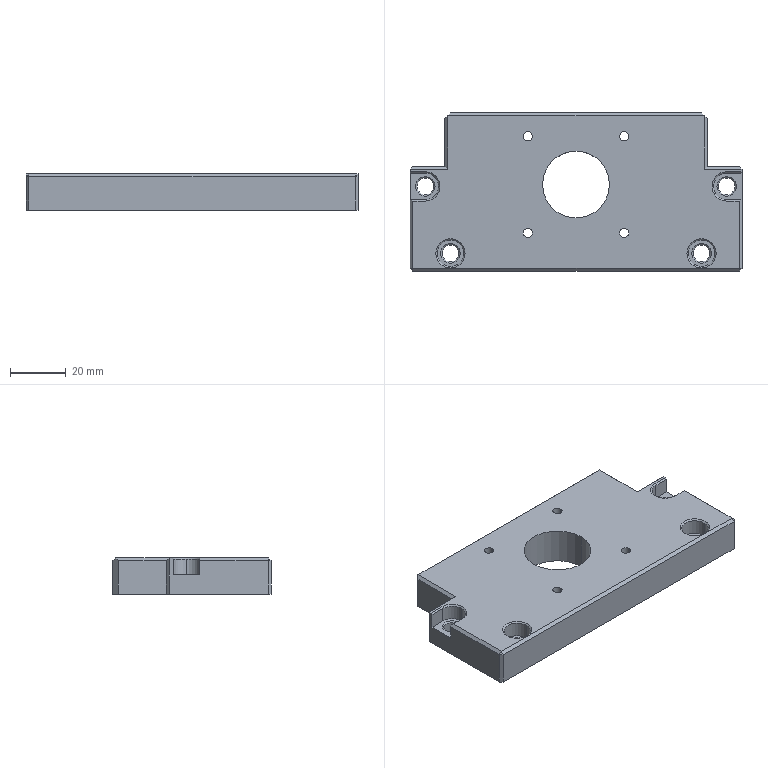Part | STEP file | LES120 bearing housing^FTH120-PD-direct-drive motor | 1 solid | 83 faces | box 119 x 56.7 x 13 mm | volume 72115 mm3 | plane 40 | cylinder 29 | cone 14 | commonest cylinder face diameters 3.3 x8 6 x8 9.5 x7 2.5 x4 24 x2